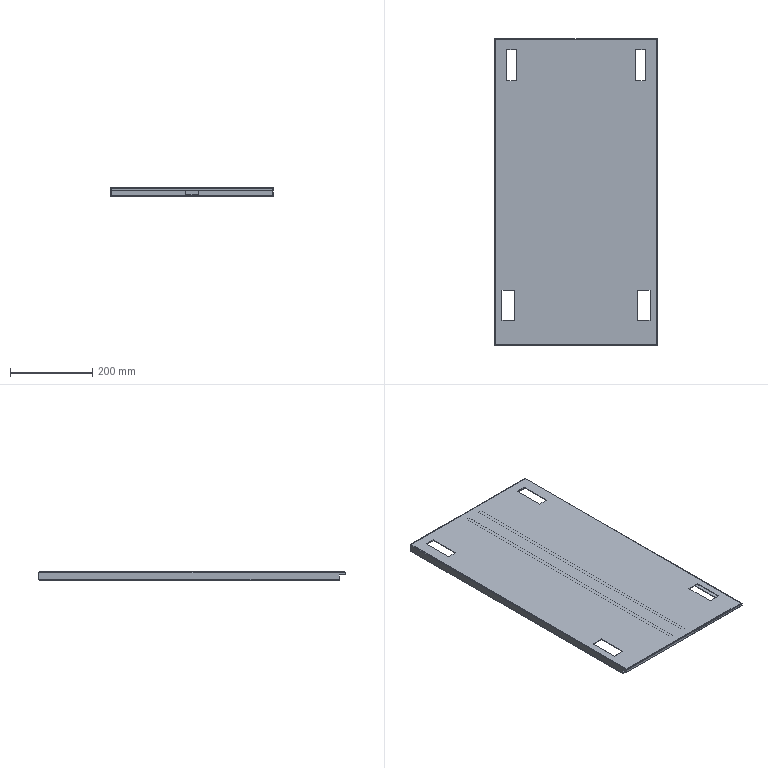Part | STEP file | FBDS-BJ-008 | 2 solids | 136 faces | box 396 x 746 x 20 mm | volume 589557 mm3 | plane 102 | cylinder 22 | spline 12 | commonest cylinder face diameters 0.4 x11 3.4 x11